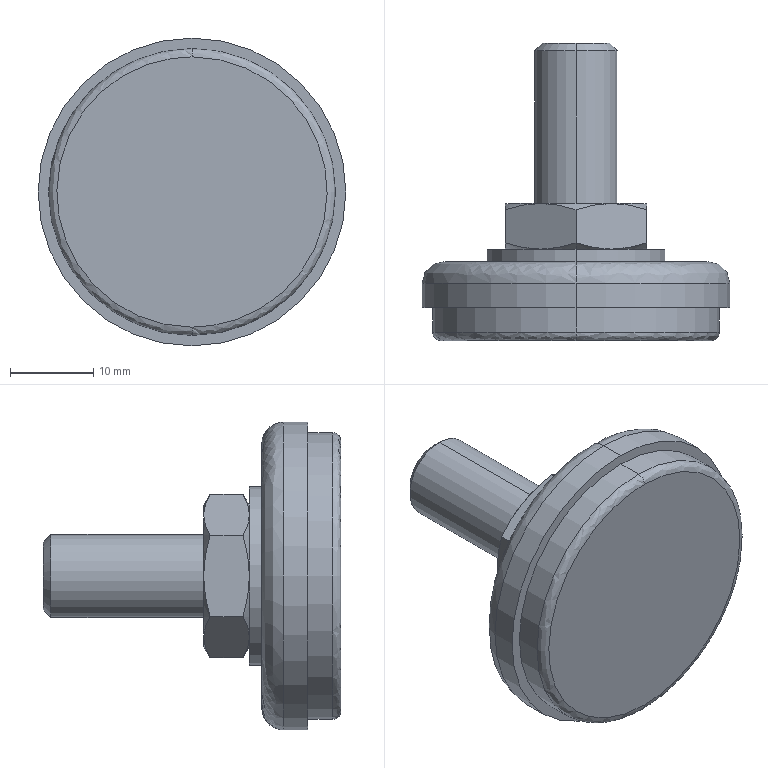Part | STEP file | _CMAZ40-N_a | 1 solid | 39 faces | box 37 x 35.8 x 37 mm | volume 12881 mm3 | cone 15 | plane 12 | cylinder 8 | spline 4 | commonest cylinder face diameters 10 x2 21.5 x2 34.5 x2 37 x2
STEP:
#1=CARTESIAN_POINT('',(0.,-15.5,17.25));
#2=VERTEX_POINT('',#1);
#3=CARTESIAN_POINT('',(0.,-15.5,-17.25));
#4=VERTEX_POINT('',#3);
#5=CARTESIAN_POINT('',(0.,-15.5,0.));
#6=DIRECTION('',(0.,-1.,0.));
#7=DIRECTION('',(0.,0.,1.));
#8=AXIS2_PLACEMENT_3D('',#5,#6,#7);
#9=CIRCLE('',#8,17.25);
#10=EDGE_CURVE('',#2,#4,#9,.T.);
#11=ORIENTED_EDGE('',*,*,#10,.T.);
#12=CARTESIAN_POINT('',(0.,-16.5,-16.25));
#13=VERTEX_POINT('',#12);
#14=CARTESIAN_POINT('',(0.,-15.5,-16.25));
#15=DIRECTION('',(-1.,0.,0.));
#16=DIRECTION('',(0.,0.,-1.));
#17=AXIS2_PLACEMENT_3D('',#14,#15,#16);
#18=CIRCLE('',#17,1.);
#19=EDGE_CURVE('',#4,#13,#18,.T.);
#20=ORIENTED_EDGE('',*,*,#19,.T.);
#21=CARTESIAN_POINT('',(0.,-16.5,16.25));
#22=VERTEX_POINT('',#21);
#23=CARTESIAN_POINT('',(0.,-16.5,-16.25));
#24=CARTESIAN_POINT('',(-32.5,-16.5,-16.25));
#25=CARTESIAN_POINT('',(-32.5,-16.5,16.25));
#26=CARTESIAN_POINT('',(0.,-16.5,16.25));
#27=(BOUNDED_CURVE()B_SPLINE_CURVE(3,(#23,#24,#25,#26),.UNSPECIFIED.,.F.,.F.)B_SPLINE_CURVE_WITH_KNOTS((4,4),(0.5,1.),.UNSPECIFIED.)CURVE()GEOMETRIC_REPRESENTATION_ITEM()RATIONAL_B_SPLINE_CURVE((1.,0.3333,0.3333,1.))REPRESENTATION_ITEM(''));
#28=EDGE_CURVE('',#13,#22,#27,.T.);
#29=ORIENTED_EDGE('',*,*,#28,.T.);
#30=CARTESIAN_POINT('',(0.,-15.5,16.25));
#31=DIRECTION('',(1.,0.,0.));
#32=DIRECTION('',(0.,0.,1.));
#33=AXIS2_PLACEMENT_3D('',#30,#31,#32);
#34=CIRCLE('',#33,1.);
#35=EDGE_CURVE('',#2,#22,#34,.T.);
#36=ORIENTED_EDGE('',*,*,#35,.F.);
#37=EDGE_LOOP('',(#11,#20,#29,#36));
#38=FACE_OUTER_BOUND('',#37,.T.);
#39=CARTESIAN_POINT('',(0.,-15.5,-17.25));
#40=CARTESIAN_POINT('',(-34.5,-15.5,-17.25));
#41=CARTESIAN_POINT('',(-34.5,-15.5,17.25));
#42=CARTESIAN_POINT('',(0.,-15.5,17.25));
#43=CARTESIAN_POINT('',(0.,-16.086,-17.25));
#44=CARTESIAN_POINT('',(-34.5,-16.086,-17.25));
#45=CARTESIAN_POINT('',(-34.5,-16.086,17.25));
#46=CARTESIAN_POINT('',(0.,-16.086,17.25));
#47=CARTESIAN_POINT('',(0.,-16.5,-16.836));
#48=CARTESIAN_POINT('',(-33.672,-16.5,-16.836));
#49=CARTESIAN_POINT('',(-33.672,-16.5,16.836));
#50=CARTESIAN_POINT('',(0.,-16.5,16.836));
#51=CARTESIAN_POINT('',(0.,-16.5,-16.25));
#52=CARTESIAN_POINT('',(-32.5,-16.5,-16.25));
#53=CARTESIAN_POINT('',(-32.5,-16.5,16.25));
#54=CARTESIAN_POINT('',(0.,-16.5,16.25));
#55=(BOUNDED_SURFACE()B_SPLINE_SURFACE(3,3,((#39,#40,#41,#42),(#43,#44,#45,#46),(#47,#48,#49,#50),(#51,#52,#53,#54)),.UNSPECIFIED.,.F.,.F.,.T.)B_SPLINE_SURFACE_WITH_KNOTS((4,4),(4,4),(0.,1.),(0.,1.),.UNSPECIFIED.)GEOMETRIC_REPRESENTATION_ITEM()RATIONAL_B_SPLINE_SURFACE(((1.,0.3333,0.3333,1.),(0.8047,0.2682,0.2682,0.8047),(0.8047,0.2682,0.2682,0.8047),(1.,0.3333,0.3333,1.)))REPRESENTATION_ITEM('')SURFACE());
#56=ADVANCED_FACE('',(#38),#55,.T.);
#57=CARTESIAN_POINT('',(0.,-7.,15.9));
#58=VERTEX_POINT('',#57);
#59=CARTESIAN_POINT('',(0.,-7.,-15.9));
#60=VERTEX_POINT('',#59);
#61=CARTESIAN_POINT('',(0.,-7.,15.9));
#62=CARTESIAN_POINT('',(-31.8,-7.,15.9));
#63=CARTESIAN_POINT('',(-31.8,-7.,-15.9));
#64=CARTESIAN_POINT('',(0.,-7.,-15.9));
#65=(BOUNDED_CURVE()B_SPLINE_CURVE(3,(#61,#62,#63,#64),.UNSPECIFIED.,.F.,.T.)B_SPLINE_CURVE_WITH_KNOTS((4,4),(0.,0.5),.UNSPECIFIED.)CURVE()GEOMETRIC_REPRESENTATION_ITEM()RATIONAL_B_SPLINE_CURVE((1.,0.3333,0.3333,1.))REPRESENTATION_ITEM(''));
#66=EDGE_CURVE('',#58,#60,#65,.T.);
#67=ORIENTED_EDGE('',*,*,#66,.T.);
#68=CARTESIAN_POINT('',(0.,-9.6,-18.5));
#69=VERTEX_POINT('',#68);
#70=CARTESIAN_POINT('',(0.,-9.6,-15.9));
#71=DIRECTION('',(-1.,0.,0.));
#72=DIRECTION('',(0.,0.,-1.));
#73=AXIS2_PLACEMENT_3D('',#70,#71,#72);
#74=CIRCLE('',#73,2.6);
#75=EDGE_CURVE('',#60,#69,#74,.T.);
#76=ORIENTED_EDGE('',*,*,#75,.T.);
#77=CARTESIAN_POINT('',(0.,-9.6,18.5));
#78=VERTEX_POINT('',#77);
#79=CARTESIAN_POINT('',(0.,-9.6,0.));
#80=DIRECTION('',(0.,-1.,0.));
#81=DIRECTION('',(0.,0.,-1.));
#82=AXIS2_PLACEMENT_3D('',#79,#80,#81);
#83=CIRCLE('',#82,18.5);
#84=EDGE_CURVE('',#78,#69,#83,.T.);
#85=ORIENTED_EDGE('',*,*,#84,.F.);
#86=CARTESIAN_POINT('',(0.,-9.6,15.9));
#87=DIRECTION('',(1.,0.,0.));
#88=DIRECTION('',(0.,0.,1.));
#89=AXIS2_PLACEMENT_3D('',#86,#87,#88);
#90=CIRCLE('',#89,2.6);
#91=EDGE_CURVE('',#58,#78,#90,.T.);
#92=ORIENTED_EDGE('',*,*,#91,.F.);
#93=EDGE_LOOP('',(#67,#76,#85,#92));
#94=FACE_OUTER_BOUND('',#93,.T.);
#95=CARTESIAN_POINT('',(0.,-7.,-15.9));
#96=CARTESIAN_POINT('',(-31.8,-7.,-15.9));
#97=CARTESIAN_POINT('',(-31.8,-7.,15.9));
#98=CARTESIAN_POINT('',(0.,-7.,15.9));
#99=CARTESIAN_POINT('',(0.,-7.,-17.423));
#100=CARTESIAN_POINT('',(-34.846,-7.,-17.423));
#101=CARTESIAN_POINT('',(-34.846,-7.,17.423));
#102=CARTESIAN_POINT('',(0.,-7.,17.423));
#103=CARTESIAN_POINT('',(0.,-8.077,-18.5));
#104=CARTESIAN_POINT('',(-37.,-8.077,-18.5));
#105=CARTESIAN_POINT('',(-37.,-8.077,18.5));
#106=CARTESIAN_POINT('',(0.,-8.077,18.5));
#107=CARTESIAN_POINT('',(0.,-9.6,-18.5));
#108=CARTESIAN_POINT('',(-37.,-9.6,-18.5));
#109=CARTESIAN_POINT('',(-37.,-9.6,18.5));
#110=CARTESIAN_POINT('',(0.,-9.6,18.5));
#111=(BOUNDED_SURFACE()B_SPLINE_SURFACE(3,3,((#95,#96,#97,#98),(#99,#100,#101,#102),(#103,#104,#105,#106),(#107,#108,#109,#110)),.UNSPECIFIED.,.F.,.F.,.F.)B_SPLINE_SURFACE_WITH_KNOTS((4,4),(4,4),(0.,1.),(0.,1.),.UNSPECIFIED.)GEOMETRIC_REPRESENTATION_ITEM()RATIONAL_B_SPLINE_SURFACE(((1.,0.3333,0.3333,1.),(0.8047,0.2682,0.2682,0.8047),(0.8047,0.2682,0.2682,0.8047),(1.,0.3333,0.3333,1.)))REPRESENTATION_ITEM('')SURFACE());
#112=ADVANCED_FACE('',(#94),#111,.T.);
#113=CARTESIAN_POINT('',(0.,-12.5,-17.25));
#114=VERTEX_POINT('',#113);
#115=CARTESIAN_POINT('',(0.,-12.5,17.25));
#116=VERTEX_POINT('',#115);
#117=CARTESIAN_POINT('',(0.,-12.5,0.));
#118=DIRECTION('',(0.,-1.,0.));
#119=DIRECTION('',(0.,0.,-1.));
#120=AXIS2_PLACEMENT_3D('',#117,#118,#119);
#121=CIRCLE('',#120,17.25);
#122=EDGE_CURVE('',#114,#116,#121,.T.);
#123=ORIENTED_EDGE('',*,*,#122,.T.);
#124=CARTESIAN_POINT('',(0.,-5.5,17.25));
#125=DIRECTION('',(0.,-1.,0.));
#126=VECTOR('',#125,1000.);
#127=LINE('',#124,#126);
#128=EDGE_CURVE('',#116,#2,#127,.T.);
#129=ORIENTED_EDGE('',*,*,#128,.T.);
#130=CARTESIAN_POINT('',(0.,-15.5,0.));
#131=DIRECTION('',(0.,-1.,0.));
#132=DIRECTION('',(0.,0.,1.));
#133=AXIS2_PLACEMENT_3D('',#130,#131,#132);
#134=CIRCLE('',#133,17.25);
#135=EDGE_CURVE('',#4,#2,#134,.T.);
#136=ORIENTED_EDGE('',*,*,#135,.F.);
#137=CARTESIAN_POINT('',(0.,-5.5,-17.25));
#138=DIRECTION('',(0.,-1.,0.));
#139=VECTOR('',#138,1000.);
#140=LINE('',#137,#139);
#141=EDGE_CURVE('',#114,#4,#140,.T.);
#142=ORIENTED_EDGE('',*,*,#141,.F.);
#143=EDGE_LOOP('',(#123,#129,#136,#142));
#144=FACE_OUTER_BOUND('',#143,.T.);
#145=CARTESIAN_POINT('',(0.,-5.5,0.));
#146=DIRECTION('',(0.,-1.,0.));
#147=DIRECTION('',(0.,0.,-1.));
#148=AXIS2_PLACEMENT_3D('',#145,#146,#147);
#149=CYLINDRICAL_SURFACE('',#148,17.25);
#150=ADVANCED_FACE('',(#144),#149,.T.);
#151=CARTESIAN_POINT('',(0.,-9.6,0.));
#152=DIRECTION('',(0.,-1.,0.));
#153=DIRECTION('',(0.,0.,-1.));
#154=AXIS2_PLACEMENT_3D('',#151,#152,#153);
#155=CIRCLE('',#154,18.5);
#156=EDGE_CURVE('',#69,#78,#155,.T.);
#157=ORIENTED_EDGE('',*,*,#156,.T.);
#158=CARTESIAN_POINT('',(0.,-12.5,18.5));
#159=VERTEX_POINT('',#158);
#160=CARTESIAN_POINT('',(0.,-5.5,18.5));
#161=DIRECTION('',(0.,-1.,0.));
#162=VECTOR('',#161,1000.);
#163=LINE('',#160,#162);
#164=EDGE_CURVE('',#78,#159,#163,.T.);
#165=ORIENTED_EDGE('',*,*,#164,.T.);
#166=CARTESIAN_POINT('',(0.,-12.5,-18.5));
#167=VERTEX_POINT('',#166);
#168=CARTESIAN_POINT('',(0.,-12.5,0.));
#169=DIRECTION('',(0.,1.,0.));
#170=DIRECTION('',(0.,0.,-1.));
#171=AXIS2_PLACEMENT_3D('',#168,#169,#170);
#172=CIRCLE('',#171,18.5);
#173=EDGE_CURVE('',#159,#167,#172,.T.);
#174=ORIENTED_EDGE('',*,*,#173,.T.);
#175=CARTESIAN_POINT('',(0.,-5.5,-18.5));
#176=DIRECTION('',(0.,-1.,0.));
#177=VECTOR('',#176,1000.);
#178=LINE('',#175,#177);
#179=EDGE_CURVE('',#69,#167,#178,.T.);
#180=ORIENTED_EDGE('',*,*,#179,.F.);
#181=EDGE_LOOP('',(#157,#165,#174,#180));
#182=FACE_OUTER_BOUND('',#181,.T.);
#183=CARTESIAN_POINT('',(0.,-5.5,0.));
#184=DIRECTION('',(0.,-1.,0.));
#185=DIRECTION('',(0.,0.,-1.));
#186=AXIS2_PLACEMENT_3D('',#183,#184,#185);
#187=CYLINDRICAL_SURFACE('',#186,18.5);
#188=ADVANCED_FACE('',(#182),#187,.T.);
#189=CARTESIAN_POINT('',(0.,-5.5,-10.75));
#190=VERTEX_POINT('',#189);
#191=CARTESIAN_POINT('',(0.,-5.5,10.75));
#192=VERTEX_POINT('',#191);
#193=CARTESIAN_POINT('',(0.,-5.5,0.));
#194=DIRECTION('',(0.,-1.,0.));
#195=DIRECTION('',(0.,0.,-1.));
#196=AXIS2_PLACEMENT_3D('',#193,#194,#195);
#197=CIRCLE('',#196,10.75);
#198=EDGE_CURVE('',#190,#192,#197,.T.);
#199=ORIENTED_EDGE('',*,*,#198,.T.);
#200=CARTESIAN_POINT('',(0.,-7.,10.75));
#201=VERTEX_POINT('',#200);
#202=CARTESIAN_POINT('',(0.,-5.5,10.75));
#203=DIRECTION('',(0.,-1.,0.));
#204=VECTOR('',#203,1000.);
#205=LINE('',#202,#204);
#206=EDGE_CURVE('',#192,#201,#205,.T.);
#207=ORIENTED_EDGE('',*,*,#206,.T.);
#208=CARTESIAN_POINT('',(0.,-7.,-10.75));
#209=VERTEX_POINT('',#208);
#210=CARTESIAN_POINT('',(0.,-7.,0.));
#211=DIRECTION('',(0.,1.,0.));
#212=DIRECTION('',(0.,0.,-1.));
#213=AXIS2_PLACEMENT_3D('',#210,#211,#212);
#214=CIRCLE('',#213,10.75);
#215=EDGE_CURVE('',#201,#209,#214,.T.);
#216=ORIENTED_EDGE('',*,*,#215,.T.);
#217=CARTESIAN_POINT('',(0.,-5.5,-10.75));
#218=DIRECTION('',(0.,-1.,0.));
#219=VECTOR('',#218,1000.);
#220=LINE('',#217,#219);
#221=EDGE_CURVE('',#190,#209,#220,.T.);
#222=ORIENTED_EDGE('',*,*,#221,.F.);
#223=EDGE_LOOP('',(#199,#207,#216,#222));
#224=FACE_OUTER_BOUND('',#223,.T.);
#225=CARTESIAN_POINT('',(0.,-5.5,0.));
#226=DIRECTION('',(0.,-1.,0.));
#227=DIRECTION('',(0.,0.,-1.));
#228=AXIS2_PLACEMENT_3D('',#225,#226,#227);
#229=CYLINDRICAL_SURFACE('',#228,10.75);
#230=ADVANCED_FACE('',(#224),#229,.T.);
#231=CARTESIAN_POINT('',(-4.25,-5.5,7.361));
#232=VERTEX_POINT('',#231);
#233=CARTESIAN_POINT('',(0.,-5.5,8.5));
#234=VERTEX_POINT('',#233);
#235=CARTESIAN_POINT('',(0.,-5.5,0.));
#236=DIRECTION('',(0.,1.,0.));
#237=DIRECTION('',(0.,0.,1.));
#238=AXIS2_PLACEMENT_3D('',#235,#236,#237);
#239=CIRCLE('',#238,8.5);
#240=EDGE_CURVE('',#232,#234,#239,.T.);
#241=ORIENTED_EDGE('',*,*,#240,.T.);
#242=CARTESIAN_POINT('',(0.000000012,-4.741,9.815));
#243=VERTEX_POINT('',#242);
#244=CARTESIAN_POINT('',(0.,-4.736,9.823));
#245=DIRECTION('',(0.,0.5,0.866));
#246=VECTOR('',#245,1000.);
#247=LINE('',#244,#246);
#248=EDGE_CURVE('',#234,#243,#247,.T.);
#249=ORIENTED_EDGE('',*,*,#248,.T.);
#250=CARTESIAN_POINT('',(0.000000012,-4.741,9.815));
#251=CARTESIAN_POINT('',(-0.6943,-4.972,9.414));
#252=CARTESIAN_POINT('',(-1.394,-5.163,9.01));
#253=CARTESIAN_POINT('',(-2.809,-5.427,8.193));
#254=CARTESIAN_POINT('',(-3.525,-5.5,7.78));
#255=CARTESIAN_POINT('',(-4.25,-5.5,7.361));
#256=B_SPLINE_CURVE_WITH_KNOTS('',3,(#250,#251,#252,#253,#254,#255),.UNSPECIFIED.,.F.,.F.,(4,2,4),(0.,0.002483,0.004966),.UNSPECIFIED.);
#257=EDGE_CURVE('',#243,#232,#256,.T.);
#258=ORIENTED_EDGE('',*,*,#257,.T.);
#259=EDGE_LOOP('',(#241,#249,#258));
#260=FACE_OUTER_BOUND('',#259,.T.);
#261=CARTESIAN_POINT('',(0.,-4.736,0.));
#262=DIRECTION('',(0.,1.,0.));
#263=DIRECTION('',(0.,0.,1.));
#264=AXIS2_PLACEMENT_3D('',#261,#262,#263);
#265=CONICAL_SURFACE('',#264,9.823,1.047);
#266=ADVANCED_FACE('',(#260),#265,.T.);
#267=CARTESIAN_POINT('',(0.,18.38,-5.));
#268=VERTEX_POINT('',#267);
#269=CARTESIAN_POINT('',(0.,18.38,5.));
#270=VERTEX_POINT('',#269);
#271=CARTESIAN_POINT('',(0.,18.38,0.));
#272=DIRECTION('',(0.,-1.,0.));
#273=DIRECTION('',(0.,0.,-1.));
#274=AXIS2_PLACEMENT_3D('',#271,#272,#273);
#275=CIRCLE('',#274,5.);
#276=EDGE_CURVE('',#268,#270,#275,.T.);
#277=ORIENTED_EDGE('',*,*,#276,.T.);
#278=CARTESIAN_POINT('',(0.,0.,5.));
#279=VERTEX_POINT('',#278);
#280=CARTESIAN_POINT('',(0.,19.3,5.));
#281=DIRECTION('',(0.,-1.,0.));
#282=VECTOR('',#281,1000.);
#283=LINE('',#280,#282);
#284=EDGE_CURVE('',#270,#279,#283,.T.);
#285=ORIENTED_EDGE('',*,*,#284,.T.);
#286=CARTESIAN_POINT('',(0.,0.,-5.));
#287=VERTEX_POINT('',#286);
#288=CARTESIAN_POINT('',(0.,0.,0.));
#289=DIRECTION('',(0.,-1.,0.));
#290=DIRECTION('',(0.,0.,-1.));
#291=AXIS2_PLACEMENT_3D('',#288,#289,#290);
#292=CIRCLE('',#291,5.);
#293=EDGE_CURVE('',#287,#279,#292,.T.);
#294=ORIENTED_EDGE('',*,*,#293,.F.);
#295=CARTESIAN_POINT('',(0.,19.3,-5.));
#296=DIRECTION('',(0.,-1.,0.));
#297=VECTOR('',#296,1000.);
#298=LINE('',#295,#297);
#299=EDGE_CURVE('',#268,#287,#298,.T.);
#300=ORIENTED_EDGE('',*,*,#299,.F.);
#301=EDGE_LOOP('',(#277,#285,#294,#300));
#302=FACE_OUTER_BOUND('',#301,.T.);
#303=CARTESIAN_POINT('',(0.,19.3,0.));
#304=DIRECTION('',(0.,-1.,0.));
#305=DIRECTION('',(0.,0.,-1.));
#306=AXIS2_PLACEMENT_3D('',#303,#304,#305);
#307=CYLINDRICAL_SURFACE('',#306,5.);
#308=ADVANCED_FACE('',(#302),#307,.T.);
#309=CARTESIAN_POINT('',(0.,19.3,-4.08));
#310=VERTEX_POINT('',#309);
#311=CARTESIAN_POINT('',(0.,19.3,4.08));
#312=VERTEX_POINT('',#311);
#313=CARTESIAN_POINT('',(0.,19.3,0.));
#314=DIRECTION('',(0.,-1.,0.));
#315=DIRECTION('',(0.,0.,-1.));
#316=AXIS2_PLACEMENT_3D('',#313,#314,#315);
#317=CIRCLE('',#316,4.08);
#318=EDGE_CURVE('',#310,#312,#317,.T.);
#319=ORIENTED_EDGE('',*,*,#318,.T.);
#320=CARTESIAN_POINT('',(0.,18.38,5.));
#321=DIRECTION('',(0.,-0.7071,0.7071));
#322=VECTOR('',#321,1000.);
#323=LINE('',#320,#322);
#324=EDGE_CURVE('',#312,#270,#323,.T.);
#325=ORIENTED_EDGE('',*,*,#324,.T.);
#326=ORIENTED_EDGE('',*,*,#276,.F.);
#327=CARTESIAN_POINT('',(0.,18.38,-5.));
#328=DIRECTION('',(0.,-0.7071,-0.7071));
#329=VECTOR('',#328,1000.);
#330=LINE('',#327,#329);
#331=EDGE_CURVE('',#310,#268,#330,.T.);
#332=ORIENTED_EDGE('',*,*,#331,.F.);
#333=EDGE_LOOP('',(#319,#325,#326,#332));
#334=FACE_OUTER_BOUND('',#333,.T.);
#335=CARTESIAN_POINT('',(0.,18.38,0.));
#336=DIRECTION('',(0.,-1.,0.));
#337=DIRECTION('',(0.,0.,-1.));
#338=AXIS2_PLACEMENT_3D('',#335,#336,#337);
#339=CONICAL_SURFACE('',#338,5.,0.7854);
#340=ADVANCED_FACE('',(#334),#339,.T.);
#341=CARTESIAN_POINT('',(0.,-16.5,16.25));
#342=CARTESIAN_POINT('',(32.5,-16.5,16.25));
#343=CARTESIAN_POINT('',(32.5,-16.5,-16.25));
#344=CARTESIAN_POINT('',(0.,-16.5,-16.25));
#345=(BOUNDED_CURVE()B_SPLINE_CURVE(3,(#341,#342,#343,#344),.UNSPECIFIED.,.F.,.T.)B_SPLINE_CURVE_WITH_KNOTS((4,4),(0.,0.5),.UNSPECIFIED.)CURVE()GEOMETRIC_REPRESENTATION_ITEM()RATIONAL_B_SPLINE_CURVE((1.,0.3333,0.3333,1.))REPRESENTATION_ITEM(''));
#346=EDGE_CURVE('',#22,#13,#345,.T.);
#347=ORIENTED_EDGE('',*,*,#346,.F.);
#348=ORIENTED_EDGE('',*,*,#28,.F.);
#349=EDGE_LOOP('',(#347,#348));
#350=FACE_OUTER_BOUND('',#349,.T.);
#351=CARTESIAN_POINT('',(0.,-16.5,0.));
#352=DIRECTION('',(0.,1.,0.));
#353=DIRECTION('',(0.,0.,1.));
#354=AXIS2_PLACEMENT_3D('',#351,#352,#353);
#355=PLANE('',#354);
#356=ADVANCED_FACE('',(#350),#355,.F.);
#357=ORIENTED_EDGE('',*,*,#19,.F.);
#358=ORIENTED_EDGE('',*,*,#135,.T.);
#359=ORIENTED_EDGE('',*,*,#35,.T.);
#360=ORIENTED_EDGE('',*,*,#346,.T.);
#361=EDGE_LOOP('',(#357,#358,#359,#360));
#362=FACE_OUTER_BOUND('',#361,.T.);
#363=CARTESIAN_POINT('',(0.,-15.5,17.25));
#364=CARTESIAN_POINT('',(34.5,-15.5,17.25));
#365=CARTESIAN_POINT('',(34.5,-15.5,-17.25));
#366=CARTESIAN_POINT('',(0.,-15.5,-17.25));
#367=CARTESIAN_POINT('',(0.,-16.086,17.25));
#368=CARTESIAN_POINT('',(34.5,-16.086,17.25));
#369=CARTESIAN_POINT('',(34.5,-16.086,-17.25));
#370=CARTESIAN_POINT('',(0.,-16.086,-17.25));
#371=CARTESIAN_POINT('',(0.,-16.5,16.836));
#372=CARTESIAN_POINT('',(33.672,-16.5,16.836));
#373=CARTESIAN_POINT('',(33.672,-16.5,-16.836));
#374=CARTESIAN_POINT('',(0.,-16.5,-16.836));
#375=CARTESIAN_POINT('',(0.,-16.5,16.25));
#376=CARTESIAN_POINT('',(32.5,-16.5,16.25));
#377=CARTESIAN_POINT('',(32.5,-16.5,-16.25));
#378=CARTESIAN_POINT('',(0.,-16.5,-16.25));
#379=(BOUNDED_SURFACE()B_SPLINE_SURFACE(3,3,((#363,#364,#365,#366),(#367,#368,#369,#370),(#371,#372,#373,#374),(#375,#376,#377,#378)),.UNSPECIFIED.,.F.,.F.,.T.)B_SPLINE_SURFACE_WITH_KNOTS((4,4),(4,4),(0.,1.),(0.,1.),.UNSPECIFIED.)GEOMETRIC_REPRESENTATION_ITEM()RATIONAL_B_SPLINE_SURFACE(((1.,0.3333,0.3333,1.),(0.8047,0.2682,0.2682,0.8047),(0.8047,0.2682,0.2682,0.8047),(1.,0.3333,0.3333,1.)))REPRESENTATION_ITEM('')SURFACE());
#380=ADVANCED_FACE('',(#362),#379,.T.);
#381=ORIENTED_EDGE('',*,*,#128,.F.);
#382=CARTESIAN_POINT('',(0.,-12.5,0.));
#383=DIRECTION('',(0.,-1.,0.));
#384=DIRECTION('',(0.,0.,-1.));
#385=AXIS2_PLACEMENT_3D('',#382,#383,#384);
#386=CIRCLE('',#385,17.25);
#387=EDGE_CURVE('',#116,#114,#386,.T.);
#388=ORIENTED_EDGE('',*,*,#387,.T.);
#389=ORIENTED_EDGE('',*,*,#141,.T.);
#390=ORIENTED_EDGE('',*,*,#10,.F.);
#391=EDGE_LOOP('',(#381,#388,#389,#390));
#392=FACE_OUTER_BOUND('',#391,.T.);
#393=CARTESIAN_POINT('',(0.,-5.5,0.));
#394=DIRECTION('',(0.,-1.,0.));
#395=DIRECTION('',(0.,0.,-1.));
#396=AXIS2_PLACEMENT_3D('',#393,#394,#395);
#397=CYLINDRICAL_SURFACE('',#396,17.25);
#398=ADVANCED_FACE('',(#392),#397,.T.);
#399=ORIENTED_EDGE('',*,*,#122,.F.);
#400=ORIENTED_EDGE('',*,*,#387,.F.);
#401=EDGE_LOOP('',(#399,#400));
#402=FACE_BOUND('',#401,.T.);
#403=CARTESIAN_POINT('',(0.,-12.5,0.));
#404=DIRECTION('',(0.,1.,0.));
#405=DIRECTION('',(0.,0.,-1.));
#406=AXIS2_PLACEMENT_3D('',#403,#404,#405);
#407=CIRCLE('',#406,18.5);
#408=EDGE_CURVE('',#167,#159,#407,.T.);
#409=ORIENTED_EDGE('',*,*,#408,.F.);
#410=ORIENTED_EDGE('',*,*,#173,.F.);
#411=EDGE_LOOP('',(#409,#410));
#412=FACE_OUTER_BOUND('',#411,.T.);
#413=CARTESIAN_POINT('',(-17.25,-12.5,0.));
#414=DIRECTION('',(0.,1.,0.));
#415=DIRECTION('',(0.,0.,1.));
#416=AXIS2_PLACEMENT_3D('',#413,#414,#415);
#417=PLANE('',#416);
#418=ADVANCED_FACE('',(#402,#412),#417,.F.);
#419=ORIENTED_EDGE('',*,*,#164,.F.);
#420=ORIENTED_EDGE('',*,*,#84,.T.);
#421=ORIENTED_EDGE('',*,*,#179,.T.);
#422=ORIENTED_EDGE('',*,*,#408,.T.);
#423=EDGE_LOOP('',(#419,#420,#421,#422));
#424=FACE_OUTER_BOUND('',#423,.T.);
#425=CARTESIAN_POINT('',(0.,-5.5,0.));
#426=DIRECTION('',(0.,-1.,0.));
#427=DIRECTION('',(0.,0.,-1.));
#428=AXIS2_PLACEMENT_3D('',#425,#426,#427);
#429=CYLINDRICAL_SURFACE('',#428,18.5);
#430=ADVANCED_FACE('',(#424),#429,.T.);
#431=ORIENTED_EDGE('',*,*,#75,.F.);
#432=CARTESIAN_POINT('',(0.,-7.,-15.9));
#433=CARTESIAN_POINT('',(31.8,-7.,-15.9));
#434=CARTESIAN_POINT('',(31.8,-7.,15.9));
#435=CARTESIAN_POINT('',(0.,-7.,15.9));
#436=(BOUNDED_CURVE()B_SPLINE_CURVE(3,(#432,#433,#434,#435),.UNSPECIFIED.,.F.,.T.)B_SPLINE_CURVE_WITH_KNOTS((4,4),(0.5,1.),.UNSPECIFIED.)CURVE()GEOMETRIC_REPRESENTATION_ITEM()RATIONAL_B_SPLINE_CURVE((1.,0.3333,0.3333,1.))REPRESENTATION_ITEM(''));
#437=EDGE_CURVE('',#60,#58,#436,.T.);
#438=ORIENTED_EDGE('',*,*,#437,.T.);
#439=ORIENTED_EDGE('',*,*,#91,.T.);
#440=ORIENTED_EDGE('',*,*,#156,.F.);
#441=EDGE_LOOP('',(#431,#438,#439,#440));
#442=FACE_OUTER_BOUND('',#441,.T.);
#443=CARTESIAN_POINT('',(0.,-7.,15.9));
#444=CARTESIAN_POINT('',(31.8,-7.,15.9));
#445=CARTESIAN_POINT('',(31.8,-7.,-15.9));
#446=CARTESIAN_POINT('',(0.,-7.,-15.9));
#447=CARTESIAN_POINT('',(0.,-7.,17.423));
#448=CARTESIAN_POINT('',(34.846,-7.,17.423));
#449=CARTESIAN_POINT('',(34.846,-7.,-17.423));
#450=CARTESIAN_POINT('',(0.,-7.,-17.423));
#451=CARTESIAN_POINT('',(0.,-8.077,18.5));
#452=CARTESIAN_POINT('',(37.,-8.077,18.5));
#453=CARTESIAN_POINT('',(37.,-8.077,-18.5));
#454=CARTESIAN_POINT('',(0.,-8.077,-18.5));
#455=CARTESIAN_POINT('',(0.,-9.6,18.5));
#456=CARTESIAN_POINT('',(37.,-9.6,18.5));
#457=CARTESIAN_POINT('',(37.,-9.6,-18.5));
#458=CARTESIAN_POINT('',(0.,-9.6,-18.5));
#459=(BOUNDED_SURFACE()B_SPLINE_SURFACE(3,3,((#443,#444,#445,#446),(#447,#448,#449,#450),(#451,#452,#453,#454),(#455,#456,#457,#458)),.UNSPECIFIED.,.F.,.F.,.F.)B_SPLINE_SURFACE_WITH_KNOTS((4,4),(4,4),(0.,1.),(0.,1.),.UNSPECIFIED.)GEOMETRIC_REPRESENTATION_ITEM()RATIONAL_B_SPLINE_SURFACE(((1.,0.3333,0.3333,1.),(0.8047,0.2682,0.2682,0.8047),(0.8047,0.2682,0.2682,0.8047),(1.,0.3333,0.3333,1.)))REPRESENTATION_ITEM('')SURFACE());
#460=ADVANCED_FACE('',(#442),#459,.T.);
#461=ORIENTED_EDGE('',*,*,#66,.F.);
#462=ORIENTED_EDGE('',*,*,#437,.F.);
#463=EDGE_LOOP('',(#461,#462));
#464=FACE_OUTER_BOUND('',#463,.T.);
#465=CARTESIAN_POINT('',(0.,-7.,0.));
#466=DIRECTION('',(0.,1.,0.));
#467=DIRECTION('',(0.,0.,-1.));
#468=AXIS2_PLACEMENT_3D('',#465,#466,#467);
#469=CIRCLE('',#468,10.75);
#470=EDGE_CURVE('',#209,#201,#469,.T.);
#471=ORIENTED_EDGE('',*,*,#470,.F.);
#472=ORIENTED_EDGE('',*,*,#215,.F.);
#473=EDGE_LOOP('',(#471,#472));
#474=FACE_BOUND('',#473,.T.);
#475=CARTESIAN_POINT('',(-15.9,-7.,0.));
#476=DIRECTION('',(0.,-1.,0.));
#477=DIRECTION('',(0.,0.,-1.));
#478=AXIS2_PLACEMENT_3D('',#475,#476,#477);
#479=PLANE('',#478);
#480=ADVANCED_FACE('',(#464,#474),#479,.F.);
#481=ORIENTED_EDGE('',*,*,#206,.F.);
#482=CARTESIAN_POINT('',(0.,-5.5,0.));
#483=DIRECTION('',(0.,-1.,0.));
#484=DIRECTION('',(0.,0.,-1.));
#485=AXIS2_PLACEMENT_3D('',#482,#483,#484);
#486=CIRCLE('',#485,10.75);
#487=EDGE_CURVE('',#192,#190,#486,.T.);
#488=ORIENTED_EDGE('',*,*,#487,.T.);
#489=ORIENTED_EDGE('',*,*,#221,.T.);
#490=ORIENTED_EDGE('',*,*,#470,.T.);
#491=EDGE_LOOP('',(#481,#488,#489,#490));
#492=FACE_OUTER_BOUND('',#491,.T.);
#493=CARTESIAN_POINT('',(0.,-5.5,0.));
#494=DIRECTION('',(0.,-1.,0.));
#495=DIRECTION('',(0.,0.,-1.));
#496=AXIS2_PLACEMENT_3D('',#493,#494,#495);
#497=CYLINDRICAL_SURFACE('',#496,10.75);
#498=ADVANCED_FACE('',(#492),#497,.T.);
#499=ORIENTED_EDGE('',*,*,#198,.F.);
#500=ORIENTED_EDGE('',*,*,#487,.F.);
#501=EDGE_LOOP('',(#499,#500));
#502=FACE_OUTER_BOUND('',#501,.T.);
#503=CARTESIAN_POINT('',(-4.25,-5.5,-7.361));
#504=VERTEX_POINT('',#503);
#505=CARTESIAN_POINT('',(-8.5,-5.5,0.));
#506=VERTEX_POINT('',#505);
#507=CARTESIAN_POINT('',(0.,-5.5,0.));
#508=DIRECTION('',(0.,1.,0.));
#509=DIRECTION('',(-1.,0.,0.));
#510=AXIS2_PLACEMENT_3D('',#507,#508,#509);
#511=CIRCLE('',#510,8.5);
#512=EDGE_CURVE('',#504,#506,#511,.T.);
#513=ORIENTED_EDGE('',*,*,#512,.F.);
#514=CARTESIAN_POINT('',(4.25,-5.5,-7.361));
#515=VERTEX_POINT('',#514);
#516=CARTESIAN_POINT('',(0.,-5.5,0.));
#517=DIRECTION('',(0.,1.,0.));
#518=DIRECTION('',(0.,0.,1.));
#519=AXIS2_PLACEMENT_3D('',#516,#517,#518);
#520=CIRCLE('',#519,8.5);
#521=EDGE_CURVE('',#515,#504,#520,.T.);
#522=ORIENTED_EDGE('',*,*,#521,.F.);
#523=CARTESIAN_POINT('',(8.5,-5.5,0.));
#524=VERTEX_POINT('',#523);
#525=CARTESIAN_POINT('',(0.,-5.5,0.));
#526=DIRECTION('',(0.,1.,0.));
#527=DIRECTION('',(-1.,0.,0.));
#528=AXIS2_PLACEMENT_3D('',#525,#526,#527);
#529=CIRCLE('',#528,8.5);
#530=EDGE_CURVE('',#524,#515,#529,.T.);
#531=ORIENTED_EDGE('',*,*,#530,.F.);
#532=CARTESIAN_POINT('',(4.25,-5.5,7.361));
#533=VERTEX_POINT('',#532);
#534=CARTESIAN_POINT('',(0.,-5.5,0.));
#535=DIRECTION('',(0.,1.,0.));
#536=DIRECTION('',(-1.,0.,0.));
#537=AXIS2_PLACEMENT_3D('',#534,#535,#536);
#538=CIRCLE('',#537,8.5);
#539=EDGE_CURVE('',#533,#524,#538,.T.);
#540=ORIENTED_EDGE('',*,*,#539,.F.);
#541=CARTESIAN_POINT('',(0.,-5.5,0.));
#542=DIRECTION('',(0.,1.,0.));
#543=DIRECTION('',(0.,0.,1.));
#544=AXIS2_PLACEMENT_3D('',#541,#542,#543);
#545=CIRCLE('',#544,8.5);
#546=EDGE_CURVE('',#234,#533,#545,.T.);
#547=ORIENTED_EDGE('',*,*,#546,.F.);
#548=ORIENTED_EDGE('',*,*,#240,.F.);
#549=CARTESIAN_POINT('',(0.,-5.5,0.));
#550=DIRECTION('',(0.,1.,0.));
#551=DIRECTION('',(-1.,0.,0.));
#552=AXIS2_PLACEMENT_3D('',#549,#550,#551);
#553=CIRCLE('',#552,8.5);
#554=EDGE_CURVE('',#506,#232,#553,.T.);
#555=ORIENTED_EDGE('',*,*,#554,.F.);
#556=EDGE_LOOP('',(#513,#522,#531,#540,#547,#548,#555));
#557=FACE_BOUND('',#556,.T.);
#558=CARTESIAN_POINT('',(-10.75,-5.5,0.));
#559=DIRECTION('',(0.,-1.,0.));
#560=DIRECTION('',(0.,0.,-1.));
#561=AXIS2_PLACEMENT_3D('',#558,#559,#560);
#562=PLANE('',#561);
#563=ADVANCED_FACE('',(#502,#557),#562,.F.);
#564=CARTESIAN_POINT('',(-8.5,-4.741,4.907));
#565=VERTEX_POINT('',#564);
#566=CARTESIAN_POINT('',(-8.5,-4.741,4.907));
#567=CARTESIAN_POINT('',(-8.5,-4.972,4.106));
#568=CARTESIAN_POINT('',(-8.5,-5.163,3.298));
#569=CARTESIAN_POINT('',(-8.5,-5.427,1.664));
#570=CARTESIAN_POINT('',(-8.5,-5.5,0.8375));
#571=CARTESIAN_POINT('',(-8.5,-5.5,0.));
#572=B_SPLINE_CURVE_WITH_KNOTS('',3,(#566,#567,#568,#569,#570,#571),.UNSPECIFIED.,.F.,.F.,(4,2,4),(0.,0.002483,0.004966),.UNSPECIFIED.);
#573=EDGE_CURVE('',#565,#506,#572,.T.);
#574=ORIENTED_EDGE('',*,*,#573,.T.);
#575=ORIENTED_EDGE('',*,*,#554,.T.);
#576=CARTESIAN_POINT('',(-4.25,-5.5,7.361));
#577=CARTESIAN_POINT('',(-4.975,-5.5,6.942));
#578=CARTESIAN_POINT('',(-5.691,-5.427,6.529));
#579=CARTESIAN_POINT('',(-7.106,-5.163,5.712));
#580=CARTESIAN_POINT('',(-7.806,-4.972,5.308));
#581=CARTESIAN_POINT('',(-8.5,-4.741,4.907));
#582=B_SPLINE_CURVE_WITH_KNOTS('',3,(#576,#577,#578,#579,#580,#581),.UNSPECIFIED.,.F.,.F.,(4,2,4),(0.,0.002483,0.004966),.UNSPECIFIED.);
#583=EDGE_CURVE('',#232,#565,#582,.T.);
#584=ORIENTED_EDGE('',*,*,#583,.T.);
#585=EDGE_LOOP('',(#574,#575,#584));
#586=FACE_OUTER_BOUND('',#585,.T.);
#587=CARTESIAN_POINT('',(0.,-4.736,0.));
#588=DIRECTION('',(0.,1.,0.));
#589=DIRECTION('',(-1.,0.,0.));
#590=AXIS2_PLACEMENT_3D('',#587,#588,#589);
#591=CONICAL_SURFACE('',#590,9.823,1.047);
#592=ADVANCED_FACE('',(#586),#591,.T.);
#593=CARTESIAN_POINT('',(-8.5,-4.741,-4.907));
#594=VERTEX_POINT('',#593);
#595=CARTESIAN_POINT('',(-8.5,-4.741,-4.907));
#596=CARTESIAN_POINT('',(-7.806,-4.972,-5.308));
#597=CARTESIAN_POINT('',(-7.106,-5.163,-5.712));
#598=CARTESIAN_POINT('',(-5.691,-5.427,-6.529));
#599=CARTESIAN_POINT('',(-4.975,-5.5,-6.942));
#600=CARTESIAN_POINT('',(-4.25,-5.5,-7.361));
#601=B_SPLINE_CURVE_WITH_KNOTS('',3,(#595,#596,#597,#598,#599,#600),.UNSPECIFIED.,.F.,.F.,(4,2,4),(0.,0.002483,0.004966),.UNSPECIFIED.);
#602=EDGE_CURVE('',#594,#504,#601,.T.);
#603=ORIENTED_EDGE('',*,*,#602,.T.);
#604=ORIENTED_EDGE('',*,*,#512,.T.);
#605=CARTESIAN_POINT('',(-8.5,-5.5,0.));
#606=CARTESIAN_POINT('',(-8.5,-5.5,-0.8375));
#607=CARTESIAN_POINT('',(-8.5,-5.427,-1.664));
#608=CARTESIAN_POINT('',(-8.5,-5.163,-3.298));
#609=CARTESIAN_POINT('',(-8.5,-4.972,-4.106));
#610=CARTESIAN_POINT('',(-8.5,-4.741,-4.907));
#611=B_SPLINE_CURVE_WITH_KNOTS('',3,(#605,#606,#607,#608,#609,#610),.UNSPECIFIED.,.F.,.F.,(4,2,4),(0.,0.002483,0.004966),.UNSPECIFIED.);
#612=EDGE_CURVE('',#506,#594,#611,.T.);
#613=ORIENTED_EDGE('',*,*,#612,.T.);
#614=EDGE_LOOP('',(#603,#604,#613));
#615=FACE_OUTER_BOUND('',#614,.T.);
#616=CARTESIAN_POINT('',(0.,-4.736,0.));
#617=DIRECTION('',(0.,1.,0.));
#618=DIRECTION('',(-1.,0.,0.));
#619=AXIS2_PLACEMENT_3D('',#616,#617,#618);
#620=CONICAL_SURFACE('',#619,9.823,1.047);
#621=ADVANCED_FACE('',(#615),#620,.T.);
#622=CARTESIAN_POINT('',(-0.000000038,-4.741,-9.815));
#623=VERTEX_POINT('',#622);
#624=CARTESIAN_POINT('',(-0.000000038,-4.741,-9.815));
#625=CARTESIAN_POINT('',(0.6943,-4.972,-9.414));
#626=CARTESIAN_POINT('',(1.394,-5.163,-9.01));
#627=CARTESIAN_POINT('',(2.809,-5.427,-8.193));
#628=CARTESIAN_POINT('',(3.525,-5.5,-7.78));
#629=CARTESIAN_POINT('',(4.25,-5.5,-7.361));
#630=B_SPLINE_CURVE_WITH_KNOTS('',3,(#624,#625,#626,#627,#628,#629),.UNSPECIFIED.,.F.,.F.,(4,2,4),(0.,0.002483,0.004966),.UNSPECIFIED.);
#631=EDGE_CURVE('',#623,#515,#630,.T.);
#632=ORIENTED_EDGE('',*,*,#631,.T.);
#633=ORIENTED_EDGE('',*,*,#521,.T.);
#634=CARTESIAN_POINT('',(-4.25,-5.5,-7.361));
#635=CARTESIAN_POINT('',(-3.525,-5.5,-7.78));
#636=CARTESIAN_POINT('',(-2.809,-5.427,-8.193));
#637=CARTESIAN_POINT('',(-1.394,-5.163,-9.01));
#638=CARTESIAN_POINT('',(-0.6943,-4.972,-9.414));
#639=CARTESIAN_POINT('',(-0.000000038,-4.741,-9.815));
#640=B_SPLINE_CURVE_WITH_KNOTS('',3,(#634,#635,#636,#637,#638,#639),.UNSPECIFIED.,.F.,.F.,(4,2,4),(0.,0.002483,0.004966),.UNSPECIFIED.);
#641=EDGE_CURVE('',#504,#623,#640,.T.);
#642=ORIENTED_EDGE('',*,*,#641,.T.);
#643=EDGE_LOOP('',(#632,#633,#642));
#644=FACE_OUTER_BOUND('',#643,.T.);
#645=CARTESIAN_POINT('',(0.,-4.736,0.));
#646=DIRECTION('',(0.,1.,0.));
#647=DIRECTION('',(0.,0.,1.));
#648=AXIS2_PLACEMENT_3D('',#645,#646,#647);
#649=CONICAL_SURFACE('',#648,9.823,1.047);
#650=ADVANCED_FACE('',(#644),#649,.T.);
#651=ORIENTED_EDGE('',*,*,#530,.T.);
#652=CARTESIAN_POINT('',(8.5,-4.741,-4.907));
#653=VERTEX_POINT('',#652);
#654=CARTESIAN_POINT('',(4.25,-5.5,-7.361));
#655=CARTESIAN_POINT('',(4.975,-5.5,-6.942));
#656=CARTESIAN_POINT('',(5.691,-5.427,-6.529));
#657=CARTESIAN_POINT('',(7.106,-5.163,-5.712));
#658=CARTESIAN_POINT('',(7.806,-4.972,-5.308));
#659=CARTESIAN_POINT('',(8.5,-4.741,-4.907));
#660=B_SPLINE_CURVE_WITH_KNOTS('',3,(#654,#655,#656,#657,#658,#659),.UNSPECIFIED.,.F.,.F.,(4,2,4),(0.,0.002483,0.004966),.UNSPECIFIED.);
#661=EDGE_CURVE('',#515,#653,#660,.T.);
#662=ORIENTED_EDGE('',*,*,#661,.T.);
#663=CARTESIAN_POINT('',(8.5,-4.741,-4.907));
#664=CARTESIAN_POINT('',(8.5,-4.972,-4.106));
#665=CARTESIAN_POINT('',(8.5,-5.163,-3.298));
#666=CARTESIAN_POINT('',(8.5,-5.427,-1.664));
#667=CARTESIAN_POINT('',(8.5,-5.5,-0.8375));
#668=CARTESIAN_POINT('',(8.5,-5.5,0.));
#669=B_SPLINE_CURVE_WITH_KNOTS('',3,(#663,#664,#665,#666,#667,#668),.UNSPECIFIED.,.F.,.F.,(4,2,4),(0.,0.002483,0.004966),.UNSPECIFIED.);
#670=EDGE_CURVE('',#653,#524,#669,.T.);
#671=ORIENTED_EDGE('',*,*,#670,.T.);
#672=EDGE_LOOP('',(#651,#662,#671));
#673=FACE_OUTER_BOUND('',#672,.T.);
#674=CARTESIAN_POINT('',(0.,-4.736,0.));
#675=DIRECTION('',(0.,1.,0.));
#676=DIRECTION('',(-1.,0.,0.));
#677=AXIS2_PLACEMENT_3D('',#674,#675,#676);
#678=CONICAL_SURFACE('',#677,9.823,1.047);
#679=ADVANCED_FACE('',(#673),#678,.T.);
#680=ORIENTED_EDGE('',*,*,#539,.T.);
#681=CARTESIAN_POINT('',(8.5,-4.741,4.907));
#682=VERTEX_POINT('',#681);
#683=CARTESIAN_POINT('',(8.5,-5.5,0.));
#684=CARTESIAN_POINT('',(8.5,-5.5,0.8375));
#685=CARTESIAN_POINT('',(8.5,-5.427,1.664));
#686=CARTESIAN_POINT('',(8.5,-5.163,3.298));
#687=CARTESIAN_POINT('',(8.5,-4.972,4.106));
#688=CARTESIAN_POINT('',(8.5,-4.741,4.907));
#689=B_SPLINE_CURVE_WITH_KNOTS('',3,(#683,#684,#685,#686,#687,#688),.UNSPECIFIED.,.F.,.F.,(4,2,4),(0.,0.002483,0.004966),.UNSPECIFIED.);
#690=EDGE_CURVE('',#524,#682,#689,.T.);
#691=ORIENTED_EDGE('',*,*,#690,.T.);
#692=CARTESIAN_POINT('',(8.5,-4.741,4.907));
#693=CARTESIAN_POINT('',(7.806,-4.972,5.308));
#694=CARTESIAN_POINT('',(7.106,-5.163,5.712));
#695=CARTESIAN_POINT('',(5.691,-5.427,6.529));
#696=CARTESIAN_POINT('',(4.975,-5.5,6.942));
#697=CARTESIAN_POINT('',(4.25,-5.5,7.361));
#698=B_SPLINE_CURVE_WITH_KNOTS('',3,(#692,#693,#694,#695,#696,#697),.UNSPECIFIED.,.F.,.F.,(4,2,4),(0.,0.002483,0.004966),.UNSPECIFIED.);
#699=EDGE_CURVE('',#682,#533,#698,.T.);
#700=ORIENTED_EDGE('',*,*,#699,.T.);
#701=EDGE_LOOP('',(#680,#691,#700));
#702=FACE_OUTER_BOUND('',#701,.T.);
#703=CARTESIAN_POINT('',(0.,-4.736,0.));
#704=DIRECTION('',(0.,1.,0.));
#705=DIRECTION('',(-1.,0.,0.));
#706=AXIS2_PLACEMENT_3D('',#703,#704,#705);
#707=CONICAL_SURFACE('',#706,9.823,1.047);
#708=ADVANCED_FACE('',(#702),#707,.T.);
#709=ORIENTED_EDGE('',*,*,#248,.F.);
#710=ORIENTED_EDGE('',*,*,#546,.T.);
#711=CARTESIAN_POINT('',(4.25,-5.5,7.361));
#712=CARTESIAN_POINT('',(3.525,-5.5,7.78));
#713=CARTESIAN_POINT('',(2.809,-5.427,8.193));
#714=CARTESIAN_POINT('',(1.394,-5.163,9.01));
#715=CARTESIAN_POINT('',(0.6943,-4.972,9.414));
#716=CARTESIAN_POINT('',(0.000000012,-4.741,9.815));
#717=B_SPLINE_CURVE_WITH_KNOTS('',3,(#711,#712,#713,#714,#715,#716),.UNSPECIFIED.,.F.,.F.,(4,2,4),(0.,0.002483,0.004966),.UNSPECIFIED.);
#718=EDGE_CURVE('',#533,#243,#717,.T.);
#719=ORIENTED_EDGE('',*,*,#718,.T.);
#720=EDGE_LOOP('',(#709,#710,#719));
#721=FACE_OUTER_BOUND('',#720,.T.);
#722=CARTESIAN_POINT('',(0.,-4.736,0.));
#723=DIRECTION('',(0.,1.,0.));
#724=DIRECTION('',(0.,0.,1.));
#725=AXIS2_PLACEMENT_3D('',#722,#723,#724);
#726=CONICAL_SURFACE('',#725,9.823,1.047);
#727=ADVANCED_FACE('',(#721),#726,.T.);
#728=CARTESIAN_POINT('',(-8.5,-0.7592,-4.907));
#729=VERTEX_POINT('',#728);
#730=CARTESIAN_POINT('',(-8.5,-5.5,-4.907));
#731=DIRECTION('',(0.,-1.,0.));
#732=VECTOR('',#731,1000.);
#733=LINE('',#730,#732);
#734=EDGE_CURVE('',#729,#594,#733,.T.);
#735=ORIENTED_EDGE('',*,*,#734,.T.);
#736=ORIENTED_EDGE('',*,*,#612,.F.);
#737=ORIENTED_EDGE('',*,*,#573,.F.);
#738=CARTESIAN_POINT('',(-8.5,-0.7592,4.907));
#739=VERTEX_POINT('',#738);
#740=CARTESIAN_POINT('',(-8.5,-5.5,4.907));
#741=DIRECTION('',(0.,1.,0.));
#742=VECTOR('',#741,1000.);
#743=LINE('',#740,#742);
#744=EDGE_CURVE('',#565,#739,#743,.T.);
#745=ORIENTED_EDGE('',*,*,#744,.T.);
#746=CARTESIAN_POINT('',(-8.5,0.,0.));
#747=VERTEX_POINT('',#746);
#748=CARTESIAN_POINT('',(-8.5,-0.7592,4.907));
#749=CARTESIAN_POINT('',(-8.5,-0.5278,4.106));
#750=CARTESIAN_POINT('',(-8.5,-0.3369,3.298));
#751=CARTESIAN_POINT('',(-8.5,-0.07258,1.664));
#752=CARTESIAN_POINT('',(-8.5,0.,0.8375));
#753=CARTESIAN_POINT('',(-8.5,0.,0.));
#754=B_SPLINE_CURVE_WITH_KNOTS('',3,(#748,#749,#750,#751,#752,#753),.UNSPECIFIED.,.F.,.F.,(4,2,4),(0.,0.002483,0.004966),.UNSPECIFIED.);
#755=EDGE_CURVE('',#739,#747,#754,.T.);
#756=ORIENTED_EDGE('',*,*,#755,.T.);
#757=CARTESIAN_POINT('',(-8.5,0.,0.));
#758=CARTESIAN_POINT('',(-8.5,0.,-0.8375));
#759=CARTESIAN_POINT('',(-8.5,-0.07258,-1.664));
#760=CARTESIAN_POINT('',(-8.5,-0.3369,-3.298));
#761=CARTESIAN_POINT('',(-8.5,-0.5278,-4.106));
#762=CARTESIAN_POINT('',(-8.5,-0.7592,-4.907));
#763=B_SPLINE_CURVE_WITH_KNOTS('',3,(#757,#758,#759,#760,#761,#762),.UNSPECIFIED.,.F.,.F.,(4,2,4),(0.,0.002483,0.004966),.UNSPECIFIED.);
#764=EDGE_CURVE('',#747,#729,#763,.T.);
#765=ORIENTED_EDGE('',*,*,#764,.T.);
#766=EDGE_LOOP('',(#735,#736,#737,#745,#756,#765));
#767=FACE_OUTER_BOUND('',#766,.T.);
#768=CARTESIAN_POINT('',(-8.5,-5.5,-4.907));
#769=DIRECTION('',(-1.,0.,0.));
#770=DIRECTION('',(0.,0.,1.));
#771=AXIS2_PLACEMENT_3D('',#768,#769,#770);
#772=PLANE('',#771);
#773=ADVANCED_FACE('',(#767),#772,.T.);
#774=ORIENTED_EDGE('',*,*,#744,.F.);
#775=ORIENTED_EDGE('',*,*,#583,.F.);
#776=ORIENTED_EDGE('',*,*,#257,.F.);
#777=CARTESIAN_POINT('',(0.,-0.7592,9.815));
#778=VERTEX_POINT('',#777);
#779=CARTESIAN_POINT('',(0.,-5.5,9.815));
#780=DIRECTION('',(0.,1.,0.));
#781=VECTOR('',#780,1000.);
#782=LINE('',#779,#781);
#783=EDGE_CURVE('',#243,#778,#782,.T.);
#784=ORIENTED_EDGE('',*,*,#783,.T.);
#785=CARTESIAN_POINT('',(-4.25,0.,7.361));
#786=VERTEX_POINT('',#785);
#787=CARTESIAN_POINT('',(0.,-0.7592,9.815));
#788=CARTESIAN_POINT('',(-0.6943,-0.5278,9.414));
#789=CARTESIAN_POINT('',(-1.394,-0.3369,9.01));
#790=CARTESIAN_POINT('',(-2.809,-0.07258,8.193));
#791=CARTESIAN_POINT('',(-3.525,0.,7.78));
#792=CARTESIAN_POINT('',(-4.25,0.,7.361));
#793=B_SPLINE_CURVE_WITH_KNOTS('',3,(#787,#788,#789,#790,#791,#792),.UNSPECIFIED.,.F.,.F.,(4,2,4),(0.,0.002483,0.004966),.UNSPECIFIED.);
#794=EDGE_CURVE('',#778,#786,#793,.T.);
#795=ORIENTED_EDGE('',*,*,#794,.T.);
#796=CARTESIAN_POINT('',(-4.25,0.,7.361));
#797=CARTESIAN_POINT('',(-4.975,0.,6.942));
#798=CARTESIAN_POINT('',(-5.691,-0.07258,6.529));
#799=CARTESIAN_POINT('',(-7.106,-0.3369,5.712));
#800=CARTESIAN_POINT('',(-7.806,-0.5278,5.308));
#801=CARTESIAN_POINT('',(-8.5,-0.7592,4.907));
#802=B_SPLINE_CURVE_WITH_KNOTS('',3,(#796,#797,#798,#799,#800,#801),.UNSPECIFIED.,.F.,.F.,(4,2,4),(0.,0.002483,0.004966),.UNSPECIFIED.);
#803=EDGE_CURVE('',#786,#739,#802,.T.);
#804=ORIENTED_EDGE('',*,*,#803,.T.);
#805=EDGE_LOOP('',(#774,#775,#776,#784,#795,#804));
#806=FACE_OUTER_BOUND('',#805,.T.);
#807=CARTESIAN_POINT('',(-8.5,-5.5,4.907));
#808=DIRECTION('',(-0.5,0.,0.866));
#809=DIRECTION('',(0.866,0.,0.5));
#810=AXIS2_PLACEMENT_3D('',#807,#808,#809);
#811=PLANE('',#810);
#812=ADVANCED_FACE('',(#806),#811,.T.);
#813=CARTESIAN_POINT('',(0.,-0.7592,-9.815));
#814=VERTEX_POINT('',#813);
#815=CARTESIAN_POINT('',(0.,-5.5,-9.815));
#816=DIRECTION('',(0.,-1.,0.));
#817=VECTOR('',#816,1000.);
#818=LINE('',#815,#817);
#819=EDGE_CURVE('',#814,#623,#818,.T.);
#820=ORIENTED_EDGE('',*,*,#819,.T.);
#821=ORIENTED_EDGE('',*,*,#641,.F.);
#822=ORIENTED_EDGE('',*,*,#602,.F.);
#823=ORIENTED_EDGE('',*,*,#734,.F.);
#824=CARTESIAN_POINT('',(-4.25,0.,-7.361));
#825=VERTEX_POINT('',#824);
#826=CARTESIAN_POINT('',(-8.5,-0.7592,-4.907));
#827=CARTESIAN_POINT('',(-7.806,-0.5278,-5.308));
#828=CARTESIAN_POINT('',(-7.106,-0.3369,-5.712));
#829=CARTESIAN_POINT('',(-5.691,-0.07258,-6.529));
#830=CARTESIAN_POINT('',(-4.975,0.,-6.942));
#831=CARTESIAN_POINT('',(-4.25,0.,-7.361));
#832=B_SPLINE_CURVE_WITH_KNOTS('',3,(#826,#827,#828,#829,#830,#831),.UNSPECIFIED.,.F.,.F.,(4,2,4),(0.,0.002483,0.004966),.UNSPECIFIED.);
#833=EDGE_CURVE('',#729,#825,#832,.T.);
#834=ORIENTED_EDGE('',*,*,#833,.T.);
#835=CARTESIAN_POINT('',(-4.25,0.,-7.361));
#836=CARTESIAN_POINT('',(-3.525,0.,-7.78));
#837=CARTESIAN_POINT('',(-2.809,-0.07258,-8.193));
#838=CARTESIAN_POINT('',(-1.394,-0.3369,-9.01));
#839=CARTESIAN_POINT('',(-0.6943,-0.5278,-9.414));
#840=CARTESIAN_POINT('',(0.,-0.7592,-9.815));
#841=B_SPLINE_CURVE_WITH_KNOTS('',3,(#835,#836,#837,#838,#839,#840),.UNSPECIFIED.,.F.,.F.,(4,2,4),(0.,0.002483,0.004966),.UNSPECIFIED.);
#842=EDGE_CURVE('',#825,#814,#841,.T.);
#843=ORIENTED_EDGE('',*,*,#842,.T.);
#844=EDGE_LOOP('',(#820,#821,#822,#823,#834,#843));
#845=FACE_OUTER_BOUND('',#844,.T.);
#846=CARTESIAN_POINT('',(0.,-5.5,-9.815));
#847=DIRECTION('',(-0.5,0.,-0.866));
#848=DIRECTION('',(-0.866,0.,0.5));
#849=AXIS2_PLACEMENT_3D('',#846,#847,#848);
#850=PLANE('',#849);
#851=ADVANCED_FACE('',(#845),#850,.T.);
#852=CARTESIAN_POINT('',(8.5,-0.7592,-4.907));
#853=VERTEX_POINT('',#852);
#854=CARTESIAN_POINT('',(8.5,-5.5,-4.907));
#855=DIRECTION('',(0.,-1.,0.));
#856=VECTOR('',#855,1000.);
#857=LINE('',#854,#856);
#858=EDGE_CURVE('',#853,#653,#857,.T.);
#859=ORIENTED_EDGE('',*,*,#858,.T.);
#860=ORIENTED_EDGE('',*,*,#661,.F.);
#861=ORIENTED_EDGE('',*,*,#631,.F.);
#862=ORIENTED_EDGE('',*,*,#819,.F.);
#863=CARTESIAN_POINT('',(4.25,0.,-7.361));
#864=VERTEX_POINT('',#863);
#865=CARTESIAN_POINT('',(0.,-0.7592,-9.815));
#866=CARTESIAN_POINT('',(0.6943,-0.5278,-9.414));
#867=CARTESIAN_POINT('',(1.394,-0.3369,-9.01));
#868=CARTESIAN_POINT('',(2.809,-0.07258,-8.193));
#869=CARTESIAN_POINT('',(3.525,0.,-7.78));
#870=CARTESIAN_POINT('',(4.25,0.,-7.361));
#871=B_SPLINE_CURVE_WITH_KNOTS('',3,(#865,#866,#867,#868,#869,#870),.UNSPECIFIED.,.F.,.F.,(4,2,4),(0.,0.002483,0.004966),.UNSPECIFIED.);
#872=EDGE_CURVE('',#814,#864,#871,.T.);
#873=ORIENTED_EDGE('',*,*,#872,.T.);
#874=CARTESIAN_POINT('',(4.25,0.,-7.361));
#875=CARTESIAN_POINT('',(4.975,0.,-6.942));
#876=CARTESIAN_POINT('',(5.691,-0.07258,-6.529));
#877=CARTESIAN_POINT('',(7.106,-0.3369,-5.712));
#878=CARTESIAN_POINT('',(7.806,-0.5278,-5.308));
#879=CARTESIAN_POINT('',(8.5,-0.7592,-4.907));
#880=B_SPLINE_CURVE_WITH_KNOTS('',3,(#874,#875,#876,#877,#878,#879),.UNSPECIFIED.,.F.,.F.,(4,2,4),(0.,0.002483,0.004966),.UNSPECIFIED.);
#881=EDGE_CURVE('',#864,#853,#880,.T.);
#882=ORIENTED_EDGE('',*,*,#881,.T.);
#883=EDGE_LOOP('',(#859,#860,#861,#862,#873,#882));
#884=FACE_OUTER_BOUND('',#883,.T.);
#885=CARTESIAN_POINT('',(8.5,-5.5,-4.907));
#886=DIRECTION('',(0.5,0.,-0.866));
#887=DIRECTION('',(-0.866,0.,-0.5));
#888=AXIS2_PLACEMENT_3D('',#885,#886,#887);
#889=PLANE('',#888);
#890=ADVANCED_FACE('',(#884),#889,.T.);
#891=CARTESIAN_POINT('',(8.5,-0.7592,4.907));
#892=VERTEX_POINT('',#891);
#893=CARTESIAN_POINT('',(8.5,-5.5,4.907));
#894=DIRECTION('',(0.,-1.,0.));
#895=VECTOR('',#894,1000.);
#896=LINE('',#893,#895);
#897=EDGE_CURVE('',#892,#682,#896,.T.);
#898=ORIENTED_EDGE('',*,*,#897,.T.);
#899=ORIENTED_EDGE('',*,*,#690,.F.);
#900=ORIENTED_EDGE('',*,*,#670,.F.);
#901=ORIENTED_EDGE('',*,*,#858,.F.);
#902=CARTESIAN_POINT('',(8.5,0.,0.));
#903=VERTEX_POINT('',#902);
#904=CARTESIAN_POINT('',(8.5,-0.7592,-4.907));
#905=CARTESIAN_POINT('',(8.5,-0.5278,-4.106));
#906=CARTESIAN_POINT('',(8.5,-0.3369,-3.298));
#907=CARTESIAN_POINT('',(8.5,-0.07258,-1.664));
#908=CARTESIAN_POINT('',(8.5,0.,-0.8375));
#909=CARTESIAN_POINT('',(8.5,0.,0.));
#910=B_SPLINE_CURVE_WITH_KNOTS('',3,(#904,#905,#906,#907,#908,#909),.UNSPECIFIED.,.F.,.F.,(4,2,4),(0.,0.002483,0.004966),.UNSPECIFIED.);
#911=EDGE_CURVE('',#853,#903,#910,.T.);
#912=ORIENTED_EDGE('',*,*,#911,.T.);
#913=CARTESIAN_POINT('',(8.5,0.,0.));
#914=CARTESIAN_POINT('',(8.5,0.,0.8375));
#915=CARTESIAN_POINT('',(8.5,-0.07258,1.664));
#916=CARTESIAN_POINT('',(8.5,-0.3369,3.298));
#917=CARTESIAN_POINT('',(8.5,-0.5278,4.106));
#918=CARTESIAN_POINT('',(8.5,-0.7592,4.907));
#919=B_SPLINE_CURVE_WITH_KNOTS('',3,(#913,#914,#915,#916,#917,#918),.UNSPECIFIED.,.F.,.F.,(4,2,4),(0.,0.002483,0.004966),.UNSPECIFIED.);
#920=EDGE_CURVE('',#903,#892,#919,.T.);
#921=ORIENTED_EDGE('',*,*,#920,.T.);
#922=EDGE_LOOP('',(#898,#899,#900,#901,#912,#921));
#923=FACE_OUTER_BOUND('',#922,.T.);
#924=CARTESIAN_POINT('',(8.5,-5.5,4.907));
#925=DIRECTION('',(1.,0.,0.));
#926=DIRECTION('',(0.,0.,-1.));
#927=AXIS2_PLACEMENT_3D('',#924,#925,#926);
#928=PLANE('',#927);
#929=ADVANCED_FACE('',(#923),#928,.T.);
#930=ORIENTED_EDGE('',*,*,#783,.F.);
#931=ORIENTED_EDGE('',*,*,#718,.F.);
#932=ORIENTED_EDGE('',*,*,#699,.F.);
#933=ORIENTED_EDGE('',*,*,#897,.F.);
#934=CARTESIAN_POINT('',(4.25,0.,7.361));
#935=VERTEX_POINT('',#934);
#936=CARTESIAN_POINT('',(8.5,-0.7592,4.907));
#937=CARTESIAN_POINT('',(7.806,-0.5278,5.308));
#938=CARTESIAN_POINT('',(7.106,-0.3369,5.712));
#939=CARTESIAN_POINT('',(5.691,-0.07258,6.529));
#940=CARTESIAN_POINT('',(4.975,0.,6.942));
#941=CARTESIAN_POINT('',(4.25,0.,7.361));
#942=B_SPLINE_CURVE_WITH_KNOTS('',3,(#936,#937,#938,#939,#940,#941),.UNSPECIFIED.,.F.,.F.,(4,2,4),(0.,0.002483,0.004966),.UNSPECIFIED.);
#943=EDGE_CURVE('',#892,#935,#942,.T.);
#944=ORIENTED_EDGE('',*,*,#943,.T.);
#945=CARTESIAN_POINT('',(4.25,0.,7.361));
#946=CARTESIAN_POINT('',(3.525,0.,7.78));
#947=CARTESIAN_POINT('',(2.809,-0.07258,8.193));
#948=CARTESIAN_POINT('',(1.394,-0.3369,9.01));
#949=CARTESIAN_POINT('',(0.6943,-0.5278,9.414));
#950=CARTESIAN_POINT('',(0.,-0.7592,9.815));
#951=B_SPLINE_CURVE_WITH_KNOTS('',3,(#945,#946,#947,#948,#949,#950),.UNSPECIFIED.,.F.,.F.,(4,2,4),(0.,0.002483,0.004966),.UNSPECIFIED.);
#952=EDGE_CURVE('',#935,#778,#951,.T.);
#953=ORIENTED_EDGE('',*,*,#952,.T.);
#954=EDGE_LOOP('',(#930,#931,#932,#933,#944,#953));
#955=FACE_OUTER_BOUND('',#954,.T.);
#956=CARTESIAN_POINT('',(0.,-5.5,9.815));
#957=DIRECTION('',(0.5,0.,0.866));
#958=DIRECTION('',(0.866,0.,-0.5));
#959=AXIS2_PLACEMENT_3D('',#956,#957,#958);
#960=PLANE('',#959);
#961=ADVANCED_FACE('',(#955),#960,.T.);
#962=ORIENTED_EDGE('',*,*,#764,.F.);
#963=CARTESIAN_POINT('',(0.,0.,0.));
#964=DIRECTION('',(0.,-1.,0.));
#965=DIRECTION('',(0.,0.,-1.));
#966=AXIS2_PLACEMENT_3D('',#963,#964,#965);
#967=CIRCLE('',#966,8.5);
#968=EDGE_CURVE('',#747,#825,#967,.T.);
#969=ORIENTED_EDGE('',*,*,#968,.T.);
#970=ORIENTED_EDGE('',*,*,#833,.F.);
#971=EDGE_LOOP('',(#962,#969,#970));
#972=FACE_OUTER_BOUND('',#971,.T.);
#973=CARTESIAN_POINT('',(0.,-0.7637,0.));
#974=DIRECTION('',(0.,-1.,0.));
#975=DIRECTION('',(0.,0.,-1.));
#976=AXIS2_PLACEMENT_3D('',#973,#974,#975);
#977=CONICAL_SURFACE('',#976,9.823,1.047);
#978=ADVANCED_FACE('',(#972),#977,.T.);
#979=ORIENTED_EDGE('',*,*,#803,.F.);
#980=CARTESIAN_POINT('',(0.,0.,0.));
#981=DIRECTION('',(0.,-1.,0.));
#982=DIRECTION('',(0.,0.,-1.));
#983=AXIS2_PLACEMENT_3D('',#980,#981,#982);
#984=CIRCLE('',#983,8.5);
#985=EDGE_CURVE('',#786,#747,#984,.T.);
#986=ORIENTED_EDGE('',*,*,#985,.T.);
#987=ORIENTED_EDGE('',*,*,#755,.F.);
#988=EDGE_LOOP('',(#979,#986,#987));
#989=FACE_OUTER_BOUND('',#988,.T.);
#990=CARTESIAN_POINT('',(0.,-0.7637,0.));
#991=DIRECTION('',(0.,-1.,0.));
#992=DIRECTION('',(0.,0.,-1.));
#993=AXIS2_PLACEMENT_3D('',#990,#991,#992);
#994=CONICAL_SURFACE('',#993,9.823,1.047);
#995=ADVANCED_FACE('',(#989),#994,.T.);
#996=ORIENTED_EDGE('',*,*,#952,.F.);
#997=CARTESIAN_POINT('',(0.,0.,0.));
#998=DIRECTION('',(0.,-1.,0.));
#999=DIRECTION('',(1.,0.,0.));
#1000=AXIS2_PLACEMENT_3D('',#997,#998,#999);
#1001=CIRCLE('',#1000,8.5);
#1002=EDGE_CURVE('',#935,#786,#1001,.T.);
#1003=ORIENTED_EDGE('',*,*,#1002,.T.);
#1004=ORIENTED_EDGE('',*,*,#794,.F.);
#1005=EDGE_LOOP('',(#996,#1003,#1004));
#1006=FACE_OUTER_BOUND('',#1005,.T.);
#1007=CARTESIAN_POINT('',(0.,-0.7637,0.));
#1008=DIRECTION('',(0.,-1.,0.));
#1009=DIRECTION('',(1.,0.,0.));
#1010=AXIS2_PLACEMENT_3D('',#1007,#1008,#1009);
#1011=CONICAL_SURFACE('',#1010,9.823,1.047);
#1012=ADVANCED_FACE('',(#1006),#1011,.T.);
#1013=CARTESIAN_POINT('',(0.,0.,0.));
#1014=DIRECTION('',(0.,-1.,0.));
#1015=DIRECTION('',(1.,0.,0.));
#1016=AXIS2_PLACEMENT_3D('',#1013,#1014,#1015);
#1017=CIRCLE('',#1016,8.5);
#1018=EDGE_CURVE('',#825,#864,#1017,.T.);
#1019=ORIENTED_EDGE('',*,*,#1018,.T.);
#1020=ORIENTED_EDGE('',*,*,#872,.F.);
#1021=ORIENTED_EDGE('',*,*,#842,.F.);
#1022=EDGE_LOOP('',(#1019,#1020,#1021));
#1023=FACE_OUTER_BOUND('',#1022,.T.);
#1024=CARTESIAN_POINT('',(0.,-0.7637,0.));
#1025=DIRECTION('',(0.,-1.,0.));
#1026=DIRECTION('',(1.,0.,0.));
#1027=AXIS2_PLACEMENT_3D('',#1024,#1025,#1026);
#1028=CONICAL_SURFACE('',#1027,9.823,1.047);
#1029=ADVANCED_FACE('',(#1023),#1028,.T.);
#1030=ORIENTED_EDGE('',*,*,#881,.F.);
#1031=CARTESIAN_POINT('',(0.,0.,0.));
#1032=DIRECTION('',(0.,-1.,0.));
#1033=DIRECTION('',(0.,0.,-1.));
#1034=AXIS2_PLACEMENT_3D('',#1031,#1032,#1033);
#1035=CIRCLE('',#1034,8.5);
#1036=EDGE_CURVE('',#864,#903,#1035,.T.);
#1037=ORIENTED_EDGE('',*,*,#1036,.T.);
#1038=ORIENTED_EDGE('',*,*,#911,.F.);
#1039=EDGE_LOOP('',(#1030,#1037,#1038));
#1040=FACE_OUTER_BOUND('',#1039,.T.);
#1041=CARTESIAN_POINT('',(0.,-0.7637,0.));
#1042=DIRECTION('',(0.,-1.,0.));
#1043=DIRECTION('',(0.,0.,-1.));
#1044=AXIS2_PLACEMENT_3D('',#1041,#1042,#1043);
#1045=CONICAL_SURFACE('',#1044,9.823,1.047);
#1046=ADVANCED_FACE('',(#1040),#1045,.T.);
#1047=ORIENTED_EDGE('',*,*,#920,.F.);
#1048=CARTESIAN_POINT('',(0.,0.,0.));
#1049=DIRECTION('',(0.,-1.,0.));
#1050=DIRECTION('',(0.,0.,-1.));
#1051=AXIS2_PLACEMENT_3D('',#1048,#1049,#1050);
#1052=CIRCLE('',#1051,8.5);
#1053=EDGE_CURVE('',#903,#935,#1052,.T.);
#1054=ORIENTED_EDGE('',*,*,#1053,.T.);
#1055=ORIENTED_EDGE('',*,*,#943,.F.);
#1056=EDGE_LOOP('',(#1047,#1054,#1055));
#1057=FACE_OUTER_BOUND('',#1056,.T.);
#1058=CARTESIAN_POINT('',(0.,-0.7637,0.));
#1059=DIRECTION('',(0.,-1.,0.));
#1060=DIRECTION('',(0.,0.,-1.));
#1061=AXIS2_PLACEMENT_3D('',#1058,#1059,#1060);
#1062=CONICAL_SURFACE('',#1061,9.823,1.047);
#1063=ADVANCED_FACE('',(#1057),#1062,.T.);
#1064=ORIENTED_EDGE('',*,*,#293,.T.);
#1065=CARTESIAN_POINT('',(0.,0.,0.));
#1066=DIRECTION('',(0.,-1.,0.));
#1067=DIRECTION('',(0.,0.,-1.));
#1068=AXIS2_PLACEMENT_3D('',#1065,#1066,#1067);
#1069=CIRCLE('',#1068,5.);
#1070=EDGE_CURVE('',#279,#287,#1069,.T.);
#1071=ORIENTED_EDGE('',*,*,#1070,.T.);
#1072=EDGE_LOOP('',(#1064,#1071));
#1073=FACE_BOUND('',#1072,.T.);
#1074=ORIENTED_EDGE('',*,*,#1018,.F.);
#1075=ORIENTED_EDGE('',*,*,#968,.F.);
#1076=ORIENTED_EDGE('',*,*,#985,.F.);
#1077=ORIENTED_EDGE('',*,*,#1002,.F.);
#1078=ORIENTED_EDGE('',*,*,#1053,.F.);
#1079=ORIENTED_EDGE('',*,*,#1036,.F.);
#1080=EDGE_LOOP('',(#1074,#1075,#1076,#1077,#1078,#1079));
#1081=FACE_OUTER_BOUND('',#1080,.T.);
#1082=CARTESIAN_POINT('',(0.,0.,0.));
#1083=DIRECTION('',(0.,1.,0.));
#1084=DIRECTION('',(0.,0.,1.));
#1085=AXIS2_PLACEMENT_3D('',#1082,#1083,#1084);
#1086=PLANE('',#1085);
#1087=ADVANCED_FACE('',(#1073,#1081),#1086,.T.);
#1088=ORIENTED_EDGE('',*,*,#284,.F.);
#1089=CARTESIAN_POINT('',(0.,18.38,0.));
#1090=DIRECTION('',(0.,-1.,0.));
#1091=DIRECTION('',(0.,0.,-1.));
#1092=AXIS2_PLACEMENT_3D('',#1089,#1090,#1091);
#1093=CIRCLE('',#1092,5.);
#1094=EDGE_CURVE('',#270,#268,#1093,.T.);
#1095=ORIENTED_EDGE('',*,*,#1094,.T.);
#1096=ORIENTED_EDGE('',*,*,#299,.T.);
#1097=ORIENTED_EDGE('',*,*,#1070,.F.);
#1098=EDGE_LOOP('',(#1088,#1095,#1096,#1097));
#1099=FACE_OUTER_BOUND('',#1098,.T.);
#1100=CARTESIAN_POINT('',(0.,19.3,0.));
#1101=DIRECTION('',(0.,-1.,0.));
#1102=DIRECTION('',(0.,0.,-1.));
#1103=AXIS2_PLACEMENT_3D('',#1100,#1101,#1102);
#1104=CYLINDRICAL_SURFACE('',#1103,5.);
#1105=ADVANCED_FACE('',(#1099),#1104,.T.);
#1106=ORIENTED_EDGE('',*,*,#324,.F.);
#1107=CARTESIAN_POINT('',(0.,19.3,0.));
#1108=DIRECTION('',(0.,-1.,0.));
#1109=DIRECTION('',(0.,0.,-1.));
#1110=AXIS2_PLACEMENT_3D('',#1107,#1108,#1109);
#1111=CIRCLE('',#1110,4.08);
#1112=EDGE_CURVE('',#312,#310,#1111,.T.);
#1113=ORIENTED_EDGE('',*,*,#1112,.T.);
#1114=ORIENTED_EDGE('',*,*,#331,.T.);
#1115=ORIENTED_EDGE('',*,*,#1094,.F.);
#1116=EDGE_LOOP('',(#1106,#1113,#1114,#1115));
#1117=FACE_OUTER_BOUND('',#1116,.T.);
#1118=CARTESIAN_POINT('',(0.,18.38,0.));
#1119=DIRECTION('',(0.,-1.,0.));
#1120=DIRECTION('',(0.,0.,-1.));
#1121=AXIS2_PLACEMENT_3D('',#1118,#1119,#1120);
#1122=CONICAL_SURFACE('',#1121,5.,0.7854);
#1123=ADVANCED_FACE('',(#1117),#1122,.T.);
#1124=ORIENTED_EDGE('',*,*,#318,.F.);
#1125=ORIENTED_EDGE('',*,*,#1112,.F.);
#1126=EDGE_LOOP('',(#1124,#1125));
#1127=FACE_OUTER_BOUND('',#1126,.T.);
#1128=CARTESIAN_POINT('',(0.,19.3,4.08));
#1129=DIRECTION('',(0.,-1.,0.));
#1130=DIRECTION('',(0.,0.,-1.));
#1131=AXIS2_PLACEMENT_3D('',#1128,#1129,#1130);
#1132=PLANE('',#1131);
#1133=ADVANCED_FACE('',(#1127),#1132,.F.);
#1134=CLOSED_SHELL('',(#56,#112,#150,#188,#230,#266,#308,#340,#356,#380,#398,#418,#430,#460,#480,#498,#563,#592,#621,#650,#679,#708,#727,#773,#812,#851,#890,#929,#961,#978,#995,#1012,#1029,#1046,#1063,#1087,#1105,#1123,#1133));
#1135=MANIFOLD_SOLID_BREP('',#1134);
#1136=CARTESIAN_POINT('',(0.,0.,0.));
#1137=DIRECTION('',(0.,0.,1.));
#1138=DIRECTION('',(1.,0.,0.));
#1139=AXIS2_PLACEMENT_3D('',#1136,#1137,#1138);
#1140=(LENGTH_UNIT()NAMED_UNIT(*)SI_UNIT(.MILLI.,.METRE.));
#1141=UNCERTAINTY_MEASURE_WITH_UNIT(LENGTH_MEASURE(0.00001),#1140,'','');
#1142=(NAMED_UNIT(*)PLANE_ANGLE_UNIT()SI_UNIT($,.RADIAN.));
#1143=(NAMED_UNIT(*)SI_UNIT($,.STERADIAN.)SOLID_ANGLE_UNIT());
#1144=(GEOMETRIC_REPRESENTATION_CONTEXT(3)GLOBAL_UNCERTAINTY_ASSIGNED_CONTEXT((#1141))GLOBAL_UNIT_ASSIGNED_CONTEXT((#1140,#1142,#1143))REPRESENTATION_CONTEXT('',''));
#1145=ADVANCED_BREP_SHAPE_REPRESENTATION('',(#1135,#1139),#1144);